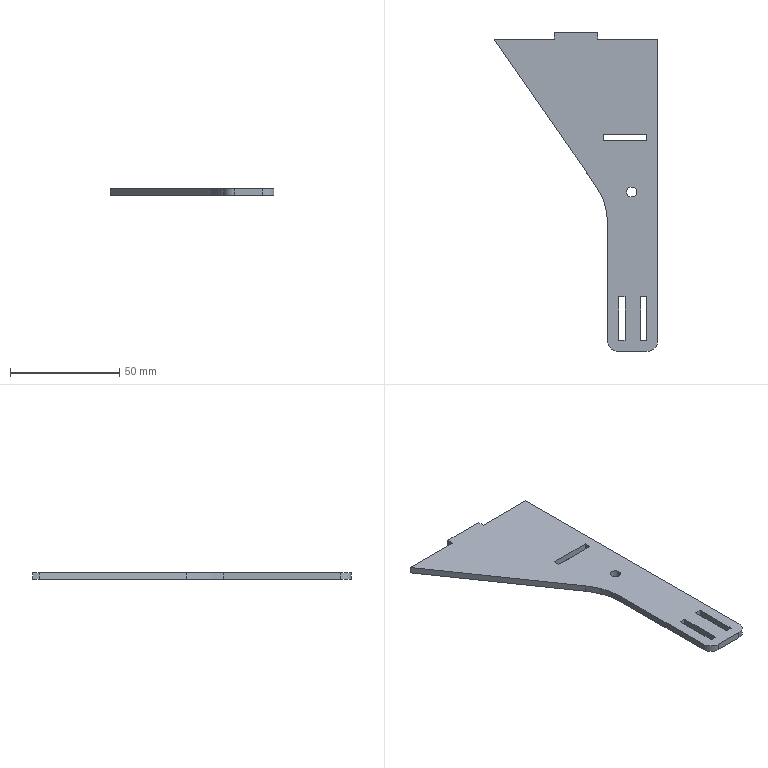Part | SolidWorks | features Fillet 2, Cut 1, Extrusion 1, ICE 1 | 1 solid | 28 faces | box 75 x 146 x 3 mm | volume 15319 mm3 | plane 23 | cylinder 5 | commonest cylinder face diameters 4.6 x2 10 x2 60 x1
STEP:
#1=CARTESIAN_POINT('',(-14.3,73.,0.));
#2=VERTEX_POINT('',#1);
#3=CARTESIAN_POINT('',(-9.7,73.,0.));
#4=VERTEX_POINT('',#3);
#5=CARTESIAN_POINT('',(-12.,73.,0.));
#6=DIRECTION('',(0.,0.,1.));
#7=DIRECTION('',(1.,0.,0.));
#8=AXIS2_PLACEMENT_3D('',#5,#6,#7);
#9=CIRCLE('',#8,2.3);
#10=EDGE_CURVE('',#2,#4,#9,.T.);
#11=ORIENTED_EDGE('',*,*,#10,.F.);
#12=CARTESIAN_POINT('',(-14.3,73.,3.));
#13=VERTEX_POINT('',#12);
#14=CARTESIAN_POINT('',(-14.3,73.,-7.));
#15=DIRECTION('',(0.,0.,1.));
#16=VECTOR('',#15,1000.);
#17=LINE('',#14,#16);
#18=EDGE_CURVE('',#2,#13,#17,.T.);
#19=ORIENTED_EDGE('',*,*,#18,.T.);
#20=CARTESIAN_POINT('',(-9.7,73.,3.));
#21=VERTEX_POINT('',#20);
#22=CARTESIAN_POINT('',(-12.,73.,3.));
#23=DIRECTION('',(0.,0.,1.));
#24=DIRECTION('',(1.,0.,0.));
#25=AXIS2_PLACEMENT_3D('',#22,#23,#24);
#26=CIRCLE('',#25,2.3);
#27=EDGE_CURVE('',#13,#21,#26,.T.);
#28=ORIENTED_EDGE('',*,*,#27,.T.);
#29=CARTESIAN_POINT('',(-9.7,73.,-7.));
#30=DIRECTION('',(0.,0.,1.));
#31=VECTOR('',#30,1000.);
#32=LINE('',#29,#31);
#33=EDGE_CURVE('',#4,#21,#32,.T.);
#34=ORIENTED_EDGE('',*,*,#33,.F.);
#35=EDGE_LOOP('',(#11,#19,#28,#34));
#36=FACE_OUTER_BOUND('',#35,.T.);
#37=CARTESIAN_POINT('',(-12.,73.,-7.));
#38=DIRECTION('',(0.,0.,1.));
#39=DIRECTION('',(1.,0.,0.));
#40=AXIS2_PLACEMENT_3D('',#37,#38,#39);
#41=CYLINDRICAL_SURFACE('',#40,2.3);
#42=ADVANCED_FACE('',(#36),#41,.F.);
#43=CARTESIAN_POINT('',(-5.,99.45,3.));
#44=VERTEX_POINT('',#43);
#45=CARTESIAN_POINT('',(-5.,96.55,3.));
#46=VERTEX_POINT('',#45);
#47=CARTESIAN_POINT('',(-5.,99.45,3.));
#48=DIRECTION('',(0.,-1.,0.));
#49=VECTOR('',#48,1000.);
#50=LINE('',#47,#49);
#51=EDGE_CURVE('',#44,#46,#50,.T.);
#52=ORIENTED_EDGE('',*,*,#51,.T.);
#53=CARTESIAN_POINT('',(-25.,96.55,3.));
#54=VERTEX_POINT('',#53);
#55=CARTESIAN_POINT('',(-5.,96.55,3.));
#56=DIRECTION('',(-1.,0.,0.));
#57=VECTOR('',#56,1000.);
#58=LINE('',#55,#57);
#59=EDGE_CURVE('',#46,#54,#58,.T.);
#60=ORIENTED_EDGE('',*,*,#59,.T.);
#61=CARTESIAN_POINT('',(-25.,99.45,3.));
#62=VERTEX_POINT('',#61);
#63=CARTESIAN_POINT('',(-25.,99.45,3.));
#64=DIRECTION('',(0.,1.,0.));
#65=VECTOR('',#64,1000.);
#66=LINE('',#63,#65);
#67=EDGE_CURVE('',#54,#62,#66,.T.);
#68=ORIENTED_EDGE('',*,*,#67,.T.);
#69=CARTESIAN_POINT('',(-5.,99.45,3.));
#70=DIRECTION('',(1.,0.,0.));
#71=VECTOR('',#70,1000.);
#72=LINE('',#69,#71);
#73=EDGE_CURVE('',#62,#44,#72,.T.);
#74=ORIENTED_EDGE('',*,*,#73,.T.);
#75=EDGE_LOOP('',(#52,#60,#68,#74));
#76=FACE_BOUND('',#75,.T.);
#77=CARTESIAN_POINT('',(-12.,73.,3.));
#78=DIRECTION('',(0.,0.,1.));
#79=DIRECTION('',(1.,0.,0.));
#80=AXIS2_PLACEMENT_3D('',#77,#78,#79);
#81=CIRCLE('',#80,2.3);
#82=EDGE_CURVE('',#21,#13,#81,.T.);
#83=ORIENTED_EDGE('',*,*,#82,.F.);
#84=ORIENTED_EDGE('',*,*,#27,.F.);
#85=EDGE_LOOP('',(#83,#84));
#86=FACE_BOUND('',#85,.T.);
#87=CARTESIAN_POINT('',(-17.95,5.,3.));
#88=VERTEX_POINT('',#87);
#89=CARTESIAN_POINT('',(-15.05,5.,3.));
#90=VERTEX_POINT('',#89);
#91=CARTESIAN_POINT('',(-17.95,5.,3.));
#92=DIRECTION('',(1.,0.,0.));
#93=VECTOR('',#92,1000.);
#94=LINE('',#91,#93);
#95=EDGE_CURVE('',#88,#90,#94,.T.);
#96=ORIENTED_EDGE('',*,*,#95,.F.);
#97=CARTESIAN_POINT('',(-17.95,25.,3.));
#98=VERTEX_POINT('',#97);
#99=CARTESIAN_POINT('',(-17.95,25.,3.));
#100=DIRECTION('',(0.,-1.,0.));
#101=VECTOR('',#100,1000.);
#102=LINE('',#99,#101);
#103=EDGE_CURVE('',#98,#88,#102,.T.);
#104=ORIENTED_EDGE('',*,*,#103,.F.);
#105=CARTESIAN_POINT('',(-15.05,25.,3.));
#106=VERTEX_POINT('',#105);
#107=CARTESIAN_POINT('',(-17.95,25.,3.));
#108=DIRECTION('',(-1.,0.,0.));
#109=VECTOR('',#108,1000.);
#110=LINE('',#107,#109);
#111=EDGE_CURVE('',#106,#98,#110,.T.);
#112=ORIENTED_EDGE('',*,*,#111,.F.);
#113=CARTESIAN_POINT('',(-15.05,25.,3.));
#114=DIRECTION('',(0.,1.,0.));
#115=VECTOR('',#114,1000.);
#116=LINE('',#113,#115);
#117=EDGE_CURVE('',#90,#106,#116,.T.);
#118=ORIENTED_EDGE('',*,*,#117,.F.);
#119=EDGE_LOOP('',(#96,#104,#112,#118));
#120=FACE_BOUND('',#119,.T.);
#121=CARTESIAN_POINT('',(-18.,0.,3.));
#122=VERTEX_POINT('',#121);
#123=CARTESIAN_POINT('',(-5.,0.,3.));
#124=VERTEX_POINT('',#123);
#125=CARTESIAN_POINT('',(0.,0.,3.));
#126=DIRECTION('',(1.,0.,0.));
#127=VECTOR('',#126,1000.);
#128=LINE('',#125,#127);
#129=EDGE_CURVE('',#122,#124,#128,.T.);
#130=ORIENTED_EDGE('',*,*,#129,.T.);
#131=CARTESIAN_POINT('',(0.,5.,3.));
#132=VERTEX_POINT('',#131);
#133=CARTESIAN_POINT('',(-5.,5.,3.));
#134=DIRECTION('',(0.,0.,1.));
#135=DIRECTION('',(1.,0.,0.));
#136=AXIS2_PLACEMENT_3D('',#133,#134,#135);
#137=CIRCLE('',#136,5.);
#138=EDGE_CURVE('',#124,#132,#137,.T.);
#139=ORIENTED_EDGE('',*,*,#138,.T.);
#140=CARTESIAN_POINT('',(0.,143.,3.));
#141=VERTEX_POINT('',#140);
#142=CARTESIAN_POINT('',(0.,0.,3.));
#143=DIRECTION('',(0.,1.,0.));
#144=VECTOR('',#143,1000.);
#145=LINE('',#142,#144);
#146=EDGE_CURVE('',#132,#141,#145,.T.);
#147=ORIENTED_EDGE('',*,*,#146,.T.);
#148=CARTESIAN_POINT('',(-27.5,143.,3.));
#149=VERTEX_POINT('',#148);
#150=CARTESIAN_POINT('',(0.,143.,3.));
#151=DIRECTION('',(-1.,0.,0.));
#152=VECTOR('',#151,1000.);
#153=LINE('',#150,#152);
#154=EDGE_CURVE('',#141,#149,#153,.T.);
#155=ORIENTED_EDGE('',*,*,#154,.T.);
#156=CARTESIAN_POINT('',(-27.5,146.,3.));
#157=VERTEX_POINT('',#156);
#158=CARTESIAN_POINT('',(-27.5,143.,3.));
#159=DIRECTION('',(0.,1.,0.));
#160=VECTOR('',#159,1000.);
#161=LINE('',#158,#160);
#162=EDGE_CURVE('',#149,#157,#161,.T.);
#163=ORIENTED_EDGE('',*,*,#162,.T.);
#164=CARTESIAN_POINT('',(-47.5,146.,3.));
#165=VERTEX_POINT('',#164);
#166=CARTESIAN_POINT('',(-47.5,146.,3.));
#167=DIRECTION('',(-1.,0.,0.));
#168=VECTOR('',#167,1000.);
#169=LINE('',#166,#168);
#170=EDGE_CURVE('',#157,#165,#169,.T.);
#171=ORIENTED_EDGE('',*,*,#170,.T.);
#172=CARTESIAN_POINT('',(-47.5,143.,3.));
#173=VERTEX_POINT('',#172);
#174=CARTESIAN_POINT('',(-47.5,143.,3.));
#175=DIRECTION('',(0.,-1.,0.));
#176=VECTOR('',#175,1000.);
#177=LINE('',#174,#176);
#178=EDGE_CURVE('',#165,#173,#177,.T.);
#179=ORIENTED_EDGE('',*,*,#178,.T.);
#180=CARTESIAN_POINT('',(-75.,143.,3.));
#181=VERTEX_POINT('',#180);
#182=CARTESIAN_POINT('',(-75.,143.,3.));
#183=DIRECTION('',(-1.,0.,0.));
#184=VECTOR('',#183,1000.);
#185=LINE('',#182,#184);
#186=EDGE_CURVE('',#173,#181,#185,.T.);
#187=ORIENTED_EDGE('',*,*,#186,.T.);
#188=CARTESIAN_POINT('',(-28.346,75.711,3.));
#189=VERTEX_POINT('',#188);
#190=CARTESIAN_POINT('',(-23.,68.,3.));
#191=DIRECTION('',(0.5698,-0.8218,0.));
#192=VECTOR('',#191,1000.);
#193=LINE('',#190,#192);
#194=EDGE_CURVE('',#181,#189,#193,.T.);
#195=ORIENTED_EDGE('',*,*,#194,.T.);
#196=CARTESIAN_POINT('',(-23.,58.617,3.));
#197=VERTEX_POINT('',#196);
#198=CARTESIAN_POINT('',(-53.,58.617,3.));
#199=DIRECTION('',(0.,0.,-1.));
#200=DIRECTION('',(1.,0.,0.));
#201=AXIS2_PLACEMENT_3D('',#198,#199,#200);
#202=CIRCLE('',#201,30.);
#203=EDGE_CURVE('',#189,#197,#202,.T.);
#204=ORIENTED_EDGE('',*,*,#203,.T.);
#205=CARTESIAN_POINT('',(-23.,5.,3.));
#206=VERTEX_POINT('',#205);
#207=CARTESIAN_POINT('',(-23.,0.,3.));
#208=DIRECTION('',(0.,-1.,0.));
#209=VECTOR('',#208,1000.);
#210=LINE('',#207,#209);
#211=EDGE_CURVE('',#197,#206,#210,.T.);
#212=ORIENTED_EDGE('',*,*,#211,.T.);
#213=CARTESIAN_POINT('',(-18.,5.,3.));
#214=DIRECTION('',(0.,0.,1.));
#215=DIRECTION('',(1.,0.,0.));
#216=AXIS2_PLACEMENT_3D('',#213,#214,#215);
#217=CIRCLE('',#216,5.);
#218=EDGE_CURVE('',#206,#122,#217,.T.);
#219=ORIENTED_EDGE('',*,*,#218,.T.);
#220=EDGE_LOOP('',(#130,#139,#147,#155,#163,#171,#179,#187,#195,#204,#212,#219));
#221=FACE_OUTER_BOUND('',#220,.T.);
#222=CARTESIAN_POINT('',(-7.95,5.,3.));
#223=VERTEX_POINT('',#222);
#224=CARTESIAN_POINT('',(-5.05,5.,3.));
#225=VERTEX_POINT('',#224);
#226=CARTESIAN_POINT('',(-7.95,5.,3.));
#227=DIRECTION('',(1.,0.,0.));
#228=VECTOR('',#227,1000.);
#229=LINE('',#226,#228);
#230=EDGE_CURVE('',#223,#225,#229,.T.);
#231=ORIENTED_EDGE('',*,*,#230,.F.);
#232=CARTESIAN_POINT('',(-7.95,25.,3.));
#233=VERTEX_POINT('',#232);
#234=CARTESIAN_POINT('',(-7.95,5.,3.));
#235=DIRECTION('',(0.,-1.,0.));
#236=VECTOR('',#235,1000.);
#237=LINE('',#234,#236);
#238=EDGE_CURVE('',#233,#223,#237,.T.);
#239=ORIENTED_EDGE('',*,*,#238,.F.);
#240=CARTESIAN_POINT('',(-5.05,25.,3.));
#241=VERTEX_POINT('',#240);
#242=CARTESIAN_POINT('',(-7.95,25.,3.));
#243=DIRECTION('',(-1.,0.,0.));
#244=VECTOR('',#243,1000.);
#245=LINE('',#242,#244);
#246=EDGE_CURVE('',#241,#233,#245,.T.);
#247=ORIENTED_EDGE('',*,*,#246,.F.);
#248=CARTESIAN_POINT('',(-5.05,5.,3.));
#249=DIRECTION('',(0.,1.,0.));
#250=VECTOR('',#249,1000.);
#251=LINE('',#248,#250);
#252=EDGE_CURVE('',#225,#241,#251,.T.);
#253=ORIENTED_EDGE('',*,*,#252,.F.);
#254=EDGE_LOOP('',(#231,#239,#247,#253));
#255=FACE_BOUND('',#254,.T.);
#256=CARTESIAN_POINT('',(0.,0.,3.));
#257=DIRECTION('',(0.,0.,1.));
#258=DIRECTION('',(1.,0.,0.));
#259=AXIS2_PLACEMENT_3D('',#256,#257,#258);
#260=PLANE('',#259);
#261=ADVANCED_FACE('',(#76,#86,#120,#221,#255),#260,.T.);
#262=CARTESIAN_POINT('',(-5.,96.55,0.));
#263=VERTEX_POINT('',#262);
#264=CARTESIAN_POINT('',(-25.,96.55,0.));
#265=VERTEX_POINT('',#264);
#266=CARTESIAN_POINT('',(-5.,96.55,0.));
#267=DIRECTION('',(-1.,0.,0.));
#268=VECTOR('',#267,1000.);
#269=LINE('',#266,#268);
#270=EDGE_CURVE('',#263,#265,#269,.T.);
#271=ORIENTED_EDGE('',*,*,#270,.F.);
#272=CARTESIAN_POINT('',(-5.,99.45,0.));
#273=VERTEX_POINT('',#272);
#274=CARTESIAN_POINT('',(-5.,99.45,0.));
#275=DIRECTION('',(0.,-1.,0.));
#276=VECTOR('',#275,1000.);
#277=LINE('',#274,#276);
#278=EDGE_CURVE('',#273,#263,#277,.T.);
#279=ORIENTED_EDGE('',*,*,#278,.F.);
#280=CARTESIAN_POINT('',(-25.,99.45,0.));
#281=VERTEX_POINT('',#280);
#282=CARTESIAN_POINT('',(-5.,99.45,0.));
#283=DIRECTION('',(1.,0.,0.));
#284=VECTOR('',#283,1000.);
#285=LINE('',#282,#284);
#286=EDGE_CURVE('',#281,#273,#285,.T.);
#287=ORIENTED_EDGE('',*,*,#286,.F.);
#288=CARTESIAN_POINT('',(-25.,99.45,0.));
#289=DIRECTION('',(0.,1.,0.));
#290=VECTOR('',#289,1000.);
#291=LINE('',#288,#290);
#292=EDGE_CURVE('',#265,#281,#291,.T.);
#293=ORIENTED_EDGE('',*,*,#292,.F.);
#294=EDGE_LOOP('',(#271,#279,#287,#293));
#295=FACE_BOUND('',#294,.T.);
#296=CARTESIAN_POINT('',(-12.,73.,0.));
#297=DIRECTION('',(0.,0.,1.));
#298=DIRECTION('',(1.,0.,0.));
#299=AXIS2_PLACEMENT_3D('',#296,#297,#298);
#300=CIRCLE('',#299,2.3);
#301=EDGE_CURVE('',#4,#2,#300,.T.);
#302=ORIENTED_EDGE('',*,*,#301,.T.);
#303=ORIENTED_EDGE('',*,*,#10,.T.);
#304=EDGE_LOOP('',(#302,#303));
#305=FACE_BOUND('',#304,.T.);
#306=CARTESIAN_POINT('',(-17.95,25.,0.));
#307=VERTEX_POINT('',#306);
#308=CARTESIAN_POINT('',(-17.95,5.,0.));
#309=VERTEX_POINT('',#308);
#310=CARTESIAN_POINT('',(-17.95,25.,0.));
#311=DIRECTION('',(0.,-1.,0.));
#312=VECTOR('',#311,1000.);
#313=LINE('',#310,#312);
#314=EDGE_CURVE('',#307,#309,#313,.T.);
#315=ORIENTED_EDGE('',*,*,#314,.T.);
#316=CARTESIAN_POINT('',(-15.05,5.,0.));
#317=VERTEX_POINT('',#316);
#318=CARTESIAN_POINT('',(-17.95,5.,0.));
#319=DIRECTION('',(1.,0.,0.));
#320=VECTOR('',#319,1000.);
#321=LINE('',#318,#320);
#322=EDGE_CURVE('',#309,#317,#321,.T.);
#323=ORIENTED_EDGE('',*,*,#322,.T.);
#324=CARTESIAN_POINT('',(-15.05,25.,0.));
#325=VERTEX_POINT('',#324);
#326=CARTESIAN_POINT('',(-15.05,25.,0.));
#327=DIRECTION('',(0.,1.,0.));
#328=VECTOR('',#327,1000.);
#329=LINE('',#326,#328);
#330=EDGE_CURVE('',#317,#325,#329,.T.);
#331=ORIENTED_EDGE('',*,*,#330,.T.);
#332=CARTESIAN_POINT('',(-17.95,25.,0.));
#333=DIRECTION('',(-1.,0.,0.));
#334=VECTOR('',#333,1000.);
#335=LINE('',#332,#334);
#336=EDGE_CURVE('',#325,#307,#335,.T.);
#337=ORIENTED_EDGE('',*,*,#336,.T.);
#338=EDGE_LOOP('',(#315,#323,#331,#337));
#339=FACE_BOUND('',#338,.T.);
#340=CARTESIAN_POINT('',(0.,5.,0.));
#341=VERTEX_POINT('',#340);
#342=CARTESIAN_POINT('',(0.,143.,0.));
#343=VERTEX_POINT('',#342);
#344=CARTESIAN_POINT('',(0.,0.,0.));
#345=DIRECTION('',(0.,1.,0.));
#346=VECTOR('',#345,1000.);
#347=LINE('',#344,#346);
#348=EDGE_CURVE('',#341,#343,#347,.T.);
#349=ORIENTED_EDGE('',*,*,#348,.F.);
#350=CARTESIAN_POINT('',(-5.,0.,0.));
#351=VERTEX_POINT('',#350);
#352=CARTESIAN_POINT('',(-5.,5.,0.));
#353=DIRECTION('',(0.,0.,-1.));
#354=DIRECTION('',(1.,0.,0.));
#355=AXIS2_PLACEMENT_3D('',#352,#353,#354);
#356=CIRCLE('',#355,5.);
#357=EDGE_CURVE('',#341,#351,#356,.T.);
#358=ORIENTED_EDGE('',*,*,#357,.T.);
#359=CARTESIAN_POINT('',(-18.,0.,0.));
#360=VERTEX_POINT('',#359);
#361=CARTESIAN_POINT('',(0.,0.,0.));
#362=DIRECTION('',(1.,0.,0.));
#363=VECTOR('',#362,1000.);
#364=LINE('',#361,#363);
#365=EDGE_CURVE('',#360,#351,#364,.T.);
#366=ORIENTED_EDGE('',*,*,#365,.F.);
#367=CARTESIAN_POINT('',(-23.,5.,0.));
#368=VERTEX_POINT('',#367);
#369=CARTESIAN_POINT('',(-18.,5.,0.));
#370=DIRECTION('',(0.,0.,-1.));
#371=DIRECTION('',(1.,0.,0.));
#372=AXIS2_PLACEMENT_3D('',#369,#370,#371);
#373=CIRCLE('',#372,5.);
#374=EDGE_CURVE('',#360,#368,#373,.T.);
#375=ORIENTED_EDGE('',*,*,#374,.T.);
#376=CARTESIAN_POINT('',(-23.,58.617,0.));
#377=VERTEX_POINT('',#376);
#378=CARTESIAN_POINT('',(-23.,0.,0.));
#379=DIRECTION('',(0.,-1.,0.));
#380=VECTOR('',#379,1000.);
#381=LINE('',#378,#380);
#382=EDGE_CURVE('',#377,#368,#381,.T.);
#383=ORIENTED_EDGE('',*,*,#382,.F.);
#384=CARTESIAN_POINT('',(-28.346,75.711,0.));
#385=VERTEX_POINT('',#384);
#386=CARTESIAN_POINT('',(-53.,58.617,0.));
#387=DIRECTION('',(0.,0.,1.));
#388=DIRECTION('',(1.,0.,0.));
#389=AXIS2_PLACEMENT_3D('',#386,#387,#388);
#390=CIRCLE('',#389,30.);
#391=EDGE_CURVE('',#377,#385,#390,.T.);
#392=ORIENTED_EDGE('',*,*,#391,.T.);
#393=CARTESIAN_POINT('',(-75.,143.,0.));
#394=VERTEX_POINT('',#393);
#395=CARTESIAN_POINT('',(-23.,68.,0.));
#396=DIRECTION('',(0.5698,-0.8218,0.));
#397=VECTOR('',#396,1000.);
#398=LINE('',#395,#397);
#399=EDGE_CURVE('',#394,#385,#398,.T.);
#400=ORIENTED_EDGE('',*,*,#399,.F.);
#401=CARTESIAN_POINT('',(-47.5,143.,0.));
#402=VERTEX_POINT('',#401);
#403=CARTESIAN_POINT('',(-75.,143.,0.));
#404=DIRECTION('',(-1.,0.,0.));
#405=VECTOR('',#404,1000.);
#406=LINE('',#403,#405);
#407=EDGE_CURVE('',#402,#394,#406,.T.);
#408=ORIENTED_EDGE('',*,*,#407,.F.);
#409=CARTESIAN_POINT('',(-47.5,146.,0.));
#410=VERTEX_POINT('',#409);
#411=CARTESIAN_POINT('',(-47.5,143.,0.));
#412=DIRECTION('',(0.,-1.,0.));
#413=VECTOR('',#412,1000.);
#414=LINE('',#411,#413);
#415=EDGE_CURVE('',#410,#402,#414,.T.);
#416=ORIENTED_EDGE('',*,*,#415,.F.);
#417=CARTESIAN_POINT('',(-27.5,146.,0.));
#418=VERTEX_POINT('',#417);
#419=CARTESIAN_POINT('',(-47.5,146.,0.));
#420=DIRECTION('',(-1.,0.,0.));
#421=VECTOR('',#420,1000.);
#422=LINE('',#419,#421);
#423=EDGE_CURVE('',#418,#410,#422,.T.);
#424=ORIENTED_EDGE('',*,*,#423,.F.);
#425=CARTESIAN_POINT('',(-27.5,143.,0.));
#426=VERTEX_POINT('',#425);
#427=CARTESIAN_POINT('',(-27.5,143.,0.));
#428=DIRECTION('',(0.,1.,0.));
#429=VECTOR('',#428,1000.);
#430=LINE('',#427,#429);
#431=EDGE_CURVE('',#426,#418,#430,.T.);
#432=ORIENTED_EDGE('',*,*,#431,.F.);
#433=CARTESIAN_POINT('',(0.,143.,0.));
#434=DIRECTION('',(-1.,0.,0.));
#435=VECTOR('',#434,1000.);
#436=LINE('',#433,#435);
#437=EDGE_CURVE('',#343,#426,#436,.T.);
#438=ORIENTED_EDGE('',*,*,#437,.F.);
#439=EDGE_LOOP('',(#349,#358,#366,#375,#383,#392,#400,#408,#416,#424,#432,#438));
#440=FACE_OUTER_BOUND('',#439,.T.);
#441=CARTESIAN_POINT('',(-7.95,25.,0.));
#442=VERTEX_POINT('',#441);
#443=CARTESIAN_POINT('',(-7.95,5.,0.));
#444=VERTEX_POINT('',#443);
#445=CARTESIAN_POINT('',(-7.95,5.,0.));
#446=DIRECTION('',(0.,-1.,0.));
#447=VECTOR('',#446,1000.);
#448=LINE('',#445,#447);
#449=EDGE_CURVE('',#442,#444,#448,.T.);
#450=ORIENTED_EDGE('',*,*,#449,.T.);
#451=CARTESIAN_POINT('',(-5.05,5.,0.));
#452=VERTEX_POINT('',#451);
#453=CARTESIAN_POINT('',(-7.95,5.,0.));
#454=DIRECTION('',(1.,0.,0.));
#455=VECTOR('',#454,1000.);
#456=LINE('',#453,#455);
#457=EDGE_CURVE('',#444,#452,#456,.T.);
#458=ORIENTED_EDGE('',*,*,#457,.T.);
#459=CARTESIAN_POINT('',(-5.05,25.,0.));
#460=VERTEX_POINT('',#459);
#461=CARTESIAN_POINT('',(-5.05,5.,0.));
#462=DIRECTION('',(0.,1.,0.));
#463=VECTOR('',#462,1000.);
#464=LINE('',#461,#463);
#465=EDGE_CURVE('',#452,#460,#464,.T.);
#466=ORIENTED_EDGE('',*,*,#465,.T.);
#467=CARTESIAN_POINT('',(-7.95,25.,0.));
#468=DIRECTION('',(-1.,0.,0.));
#469=VECTOR('',#468,1000.);
#470=LINE('',#467,#469);
#471=EDGE_CURVE('',#460,#442,#470,.T.);
#472=ORIENTED_EDGE('',*,*,#471,.T.);
#473=EDGE_LOOP('',(#450,#458,#466,#472));
#474=FACE_BOUND('',#473,.T.);
#475=CARTESIAN_POINT('',(0.,0.,0.));
#476=DIRECTION('',(0.,0.,1.));
#477=DIRECTION('',(1.,0.,0.));
#478=AXIS2_PLACEMENT_3D('',#475,#476,#477);
#479=PLANE('',#478);
#480=ADVANCED_FACE('',(#295,#305,#339,#440,#474),#479,.F.);
#481=ORIENTED_EDGE('',*,*,#146,.F.);
#482=CARTESIAN_POINT('',(0.,5.,3.));
#483=DIRECTION('',(0.,0.,-1.));
#484=VECTOR('',#483,1000.);
#485=LINE('',#482,#484);
#486=EDGE_CURVE('',#132,#341,#485,.T.);
#487=ORIENTED_EDGE('',*,*,#486,.T.);
#488=ORIENTED_EDGE('',*,*,#348,.T.);
#489=CARTESIAN_POINT('',(0.,143.,3.));
#490=DIRECTION('',(0.,0.,-1.));
#491=VECTOR('',#490,1000.);
#492=LINE('',#489,#491);
#493=EDGE_CURVE('',#141,#343,#492,.T.);
#494=ORIENTED_EDGE('',*,*,#493,.F.);
#495=EDGE_LOOP('',(#481,#487,#488,#494));
#496=FACE_OUTER_BOUND('',#495,.T.);
#497=CARTESIAN_POINT('',(0.,0.,3.));
#498=DIRECTION('',(-1.,0.,0.));
#499=DIRECTION('',(0.,0.,1.));
#500=AXIS2_PLACEMENT_3D('',#497,#498,#499);
#501=PLANE('',#500);
#502=ADVANCED_FACE('',(#496),#501,.F.);
#503=ORIENTED_EDGE('',*,*,#437,.T.);
#504=CARTESIAN_POINT('',(-27.5,143.,3.));
#505=DIRECTION('',(0.,0.,-1.));
#506=VECTOR('',#505,1000.);
#507=LINE('',#504,#506);
#508=EDGE_CURVE('',#149,#426,#507,.T.);
#509=ORIENTED_EDGE('',*,*,#508,.F.);
#510=ORIENTED_EDGE('',*,*,#154,.F.);
#511=ORIENTED_EDGE('',*,*,#493,.T.);
#512=EDGE_LOOP('',(#503,#509,#510,#511));
#513=FACE_OUTER_BOUND('',#512,.T.);
#514=CARTESIAN_POINT('',(0.,143.,3.));
#515=DIRECTION('',(0.,-1.,0.));
#516=DIRECTION('',(0.,0.,-1.));
#517=AXIS2_PLACEMENT_3D('',#514,#515,#516);
#518=PLANE('',#517);
#519=ADVANCED_FACE('',(#513),#518,.F.);
#520=ORIENTED_EDGE('',*,*,#431,.T.);
#521=CARTESIAN_POINT('',(-27.5,146.,3.));
#522=DIRECTION('',(0.,0.,-1.));
#523=VECTOR('',#522,1000.);
#524=LINE('',#521,#523);
#525=EDGE_CURVE('',#157,#418,#524,.T.);
#526=ORIENTED_EDGE('',*,*,#525,.F.);
#527=ORIENTED_EDGE('',*,*,#162,.F.);
#528=ORIENTED_EDGE('',*,*,#508,.T.);
#529=EDGE_LOOP('',(#520,#526,#527,#528));
#530=FACE_OUTER_BOUND('',#529,.T.);
#531=CARTESIAN_POINT('',(-27.5,143.,3.));
#532=DIRECTION('',(-1.,0.,0.));
#533=DIRECTION('',(0.,0.,1.));
#534=AXIS2_PLACEMENT_3D('',#531,#532,#533);
#535=PLANE('',#534);
#536=ADVANCED_FACE('',(#530),#535,.F.);
#537=ORIENTED_EDGE('',*,*,#423,.T.);
#538=CARTESIAN_POINT('',(-47.5,146.,3.));
#539=DIRECTION('',(0.,0.,-1.));
#540=VECTOR('',#539,1000.);
#541=LINE('',#538,#540);
#542=EDGE_CURVE('',#165,#410,#541,.T.);
#543=ORIENTED_EDGE('',*,*,#542,.F.);
#544=ORIENTED_EDGE('',*,*,#170,.F.);
#545=ORIENTED_EDGE('',*,*,#525,.T.);
#546=EDGE_LOOP('',(#537,#543,#544,#545));
#547=FACE_OUTER_BOUND('',#546,.T.);
#548=CARTESIAN_POINT('',(-47.5,146.,3.));
#549=DIRECTION('',(0.,-1.,0.));
#550=DIRECTION('',(0.,0.,-1.));
#551=AXIS2_PLACEMENT_3D('',#548,#549,#550);
#552=PLANE('',#551);
#553=ADVANCED_FACE('',(#547),#552,.F.);
#554=ORIENTED_EDGE('',*,*,#415,.T.);
#555=CARTESIAN_POINT('',(-47.5,143.,3.));
#556=DIRECTION('',(0.,0.,-1.));
#557=VECTOR('',#556,1000.);
#558=LINE('',#555,#557);
#559=EDGE_CURVE('',#173,#402,#558,.T.);
#560=ORIENTED_EDGE('',*,*,#559,.F.);
#561=ORIENTED_EDGE('',*,*,#178,.F.);
#562=ORIENTED_EDGE('',*,*,#542,.T.);
#563=EDGE_LOOP('',(#554,#560,#561,#562));
#564=FACE_OUTER_BOUND('',#563,.T.);
#565=CARTESIAN_POINT('',(-47.5,143.,3.));
#566=DIRECTION('',(1.,0.,0.));
#567=DIRECTION('',(0.,0.,-1.));
#568=AXIS2_PLACEMENT_3D('',#565,#566,#567);
#569=PLANE('',#568);
#570=ADVANCED_FACE('',(#564),#569,.F.);
#571=ORIENTED_EDGE('',*,*,#407,.T.);
#572=CARTESIAN_POINT('',(-75.,143.,3.));
#573=DIRECTION('',(0.,0.,-1.));
#574=VECTOR('',#573,1000.);
#575=LINE('',#572,#574);
#576=EDGE_CURVE('',#181,#394,#575,.T.);
#577=ORIENTED_EDGE('',*,*,#576,.F.);
#578=ORIENTED_EDGE('',*,*,#186,.F.);
#579=ORIENTED_EDGE('',*,*,#559,.T.);
#580=EDGE_LOOP('',(#571,#577,#578,#579));
#581=FACE_OUTER_BOUND('',#580,.T.);
#582=CARTESIAN_POINT('',(-75.,143.,3.));
#583=DIRECTION('',(0.,-1.,0.));
#584=DIRECTION('',(0.,0.,-1.));
#585=AXIS2_PLACEMENT_3D('',#582,#583,#584);
#586=PLANE('',#585);
#587=ADVANCED_FACE('',(#581),#586,.F.);
#588=ORIENTED_EDGE('',*,*,#399,.T.);
#589=CARTESIAN_POINT('',(-28.346,75.711,3.));
#590=DIRECTION('',(0.,0.,1.));
#591=VECTOR('',#590,1000.);
#592=LINE('',#589,#591);
#593=EDGE_CURVE('',#385,#189,#592,.T.);
#594=ORIENTED_EDGE('',*,*,#593,.T.);
#595=ORIENTED_EDGE('',*,*,#194,.F.);
#596=ORIENTED_EDGE('',*,*,#576,.T.);
#597=EDGE_LOOP('',(#588,#594,#595,#596));
#598=FACE_OUTER_BOUND('',#597,.T.);
#599=CARTESIAN_POINT('',(-23.,68.,3.));
#600=DIRECTION('',(0.8218,0.5698,0.));
#601=DIRECTION('',(-0.5698,0.8218,0.));
#602=AXIS2_PLACEMENT_3D('',#599,#600,#601);
#603=PLANE('',#602);
#604=ADVANCED_FACE('',(#598),#603,.F.);
#605=ORIENTED_EDGE('',*,*,#211,.F.);
#606=CARTESIAN_POINT('',(-23.,58.617,0.));
#607=DIRECTION('',(0.,0.,-1.));
#608=VECTOR('',#607,1000.);
#609=LINE('',#606,#608);
#610=EDGE_CURVE('',#197,#377,#609,.T.);
#611=ORIENTED_EDGE('',*,*,#610,.T.);
#612=ORIENTED_EDGE('',*,*,#382,.T.);
#613=CARTESIAN_POINT('',(-23.,5.,3.));
#614=DIRECTION('',(0.,0.,1.));
#615=VECTOR('',#614,1000.);
#616=LINE('',#613,#615);
#617=EDGE_CURVE('',#368,#206,#616,.T.);
#618=ORIENTED_EDGE('',*,*,#617,.T.);
#619=EDGE_LOOP('',(#605,#611,#612,#618));
#620=FACE_OUTER_BOUND('',#619,.T.);
#621=CARTESIAN_POINT('',(-23.,0.,3.));
#622=DIRECTION('',(1.,0.,0.));
#623=DIRECTION('',(0.,0.,-1.));
#624=AXIS2_PLACEMENT_3D('',#621,#622,#623);
#625=PLANE('',#624);
#626=ADVANCED_FACE('',(#620),#625,.F.);
#627=ORIENTED_EDGE('',*,*,#365,.T.);
#628=CARTESIAN_POINT('',(-5.,0.,3.));
#629=DIRECTION('',(0.,0.,1.));
#630=VECTOR('',#629,1000.);
#631=LINE('',#628,#630);
#632=EDGE_CURVE('',#351,#124,#631,.T.);
#633=ORIENTED_EDGE('',*,*,#632,.T.);
#634=ORIENTED_EDGE('',*,*,#129,.F.);
#635=CARTESIAN_POINT('',(-18.,0.,3.));
#636=DIRECTION('',(0.,0.,-1.));
#637=VECTOR('',#636,1000.);
#638=LINE('',#635,#637);
#639=EDGE_CURVE('',#122,#360,#638,.T.);
#640=ORIENTED_EDGE('',*,*,#639,.T.);
#641=EDGE_LOOP('',(#627,#633,#634,#640));
#642=FACE_OUTER_BOUND('',#641,.T.);
#643=CARTESIAN_POINT('',(0.,0.,3.));
#644=DIRECTION('',(0.,1.,0.));
#645=DIRECTION('',(0.,0.,1.));
#646=AXIS2_PLACEMENT_3D('',#643,#644,#645);
#647=PLANE('',#646);
#648=ADVANCED_FACE('',(#642),#647,.F.);
#649=ORIENTED_EDGE('',*,*,#314,.F.);
#650=CARTESIAN_POINT('',(-17.95,25.,3.));
#651=DIRECTION('',(0.,0.,-1.));
#652=VECTOR('',#651,1000.);
#653=LINE('',#650,#652);
#654=EDGE_CURVE('',#98,#307,#653,.T.);
#655=ORIENTED_EDGE('',*,*,#654,.F.);
#656=ORIENTED_EDGE('',*,*,#103,.T.);
#657=CARTESIAN_POINT('',(-17.95,5.,3.));
#658=DIRECTION('',(0.,0.,-1.));
#659=VECTOR('',#658,1000.);
#660=LINE('',#657,#659);
#661=EDGE_CURVE('',#88,#309,#660,.T.);
#662=ORIENTED_EDGE('',*,*,#661,.T.);
#663=EDGE_LOOP('',(#649,#655,#656,#662));
#664=FACE_OUTER_BOUND('',#663,.T.);
#665=CARTESIAN_POINT('',(-17.95,25.,3.));
#666=DIRECTION('',(1.,0.,0.));
#667=DIRECTION('',(0.,1.,0.));
#668=AXIS2_PLACEMENT_3D('',#665,#666,#667);
#669=PLANE('',#668);
#670=ADVANCED_FACE('',(#664),#669,.T.);
#671=ORIENTED_EDGE('',*,*,#322,.F.);
#672=ORIENTED_EDGE('',*,*,#661,.F.);
#673=ORIENTED_EDGE('',*,*,#95,.T.);
#674=CARTESIAN_POINT('',(-15.05,5.,3.));
#675=DIRECTION('',(0.,0.,-1.));
#676=VECTOR('',#675,1000.);
#677=LINE('',#674,#676);
#678=EDGE_CURVE('',#90,#317,#677,.T.);
#679=ORIENTED_EDGE('',*,*,#678,.T.);
#680=EDGE_LOOP('',(#671,#672,#673,#679));
#681=FACE_OUTER_BOUND('',#680,.T.);
#682=CARTESIAN_POINT('',(-17.95,5.,3.));
#683=DIRECTION('',(0.,1.,0.));
#684=DIRECTION('',(-1.,0.,0.));
#685=AXIS2_PLACEMENT_3D('',#682,#683,#684);
#686=PLANE('',#685);
#687=ADVANCED_FACE('',(#681),#686,.T.);
#688=ORIENTED_EDGE('',*,*,#330,.F.);
#689=ORIENTED_EDGE('',*,*,#678,.F.);
#690=ORIENTED_EDGE('',*,*,#117,.T.);
#691=CARTESIAN_POINT('',(-15.05,25.,3.));
#692=DIRECTION('',(0.,0.,-1.));
#693=VECTOR('',#692,1000.);
#694=LINE('',#691,#693);
#695=EDGE_CURVE('',#106,#325,#694,.T.);
#696=ORIENTED_EDGE('',*,*,#695,.T.);
#697=EDGE_LOOP('',(#688,#689,#690,#696));
#698=FACE_OUTER_BOUND('',#697,.T.);
#699=CARTESIAN_POINT('',(-15.05,25.,3.));
#700=DIRECTION('',(-1.,0.,0.));
#701=DIRECTION('',(0.,-1.,0.));
#702=AXIS2_PLACEMENT_3D('',#699,#700,#701);
#703=PLANE('',#702);
#704=ADVANCED_FACE('',(#698),#703,.T.);
#705=ORIENTED_EDGE('',*,*,#336,.F.);
#706=ORIENTED_EDGE('',*,*,#695,.F.);
#707=ORIENTED_EDGE('',*,*,#111,.T.);
#708=ORIENTED_EDGE('',*,*,#654,.T.);
#709=EDGE_LOOP('',(#705,#706,#707,#708));
#710=FACE_OUTER_BOUND('',#709,.T.);
#711=CARTESIAN_POINT('',(-17.95,25.,3.));
#712=DIRECTION('',(0.,-1.,0.));
#713=DIRECTION('',(1.,0.,0.));
#714=AXIS2_PLACEMENT_3D('',#711,#712,#713);
#715=PLANE('',#714);
#716=ADVANCED_FACE('',(#710),#715,.T.);
#717=ORIENTED_EDGE('',*,*,#449,.F.);
#718=CARTESIAN_POINT('',(-7.95,25.,3.));
#719=DIRECTION('',(0.,0.,-1.));
#720=VECTOR('',#719,1000.);
#721=LINE('',#718,#720);
#722=EDGE_CURVE('',#233,#442,#721,.T.);
#723=ORIENTED_EDGE('',*,*,#722,.F.);
#724=ORIENTED_EDGE('',*,*,#238,.T.);
#725=CARTESIAN_POINT('',(-7.95,5.,3.));
#726=DIRECTION('',(0.,0.,-1.));
#727=VECTOR('',#726,1000.);
#728=LINE('',#725,#727);
#729=EDGE_CURVE('',#223,#444,#728,.T.);
#730=ORIENTED_EDGE('',*,*,#729,.T.);
#731=EDGE_LOOP('',(#717,#723,#724,#730));
#732=FACE_OUTER_BOUND('',#731,.T.);
#733=CARTESIAN_POINT('',(-7.95,5.,3.));
#734=DIRECTION('',(1.,0.,0.));
#735=DIRECTION('',(0.,1.,0.));
#736=AXIS2_PLACEMENT_3D('',#733,#734,#735);
#737=PLANE('',#736);
#738=ADVANCED_FACE('',(#732),#737,.T.);
#739=ORIENTED_EDGE('',*,*,#457,.F.);
#740=ORIENTED_EDGE('',*,*,#729,.F.);
#741=ORIENTED_EDGE('',*,*,#230,.T.);
#742=CARTESIAN_POINT('',(-5.05,5.,3.));
#743=DIRECTION('',(0.,0.,-1.));
#744=VECTOR('',#743,1000.);
#745=LINE('',#742,#744);
#746=EDGE_CURVE('',#225,#452,#745,.T.);
#747=ORIENTED_EDGE('',*,*,#746,.T.);
#748=EDGE_LOOP('',(#739,#740,#741,#747));
#749=FACE_OUTER_BOUND('',#748,.T.);
#750=CARTESIAN_POINT('',(-7.95,5.,3.));
#751=DIRECTION('',(0.,1.,0.));
#752=DIRECTION('',(-1.,0.,0.));
#753=AXIS2_PLACEMENT_3D('',#750,#751,#752);
#754=PLANE('',#753);
#755=ADVANCED_FACE('',(#749),#754,.T.);
#756=ORIENTED_EDGE('',*,*,#465,.F.);
#757=ORIENTED_EDGE('',*,*,#746,.F.);
#758=ORIENTED_EDGE('',*,*,#252,.T.);
#759=CARTESIAN_POINT('',(-5.05,25.,3.));
#760=DIRECTION('',(0.,0.,-1.));
#761=VECTOR('',#760,1000.);
#762=LINE('',#759,#761);
#763=EDGE_CURVE('',#241,#460,#762,.T.);
#764=ORIENTED_EDGE('',*,*,#763,.T.);
#765=EDGE_LOOP('',(#756,#757,#758,#764));
#766=FACE_OUTER_BOUND('',#765,.T.);
#767=CARTESIAN_POINT('',(-5.05,5.,3.));
#768=DIRECTION('',(-1.,0.,0.));
#769=DIRECTION('',(0.,-1.,0.));
#770=AXIS2_PLACEMENT_3D('',#767,#768,#769);
#771=PLANE('',#770);
#772=ADVANCED_FACE('',(#766),#771,.T.);
#773=ORIENTED_EDGE('',*,*,#471,.F.);
#774=ORIENTED_EDGE('',*,*,#763,.F.);
#775=ORIENTED_EDGE('',*,*,#246,.T.);
#776=ORIENTED_EDGE('',*,*,#722,.T.);
#777=EDGE_LOOP('',(#773,#774,#775,#776));
#778=FACE_OUTER_BOUND('',#777,.T.);
#779=CARTESIAN_POINT('',(-7.95,25.,3.));
#780=DIRECTION('',(0.,-1.,0.));
#781=DIRECTION('',(0.,0.,-1.));
#782=AXIS2_PLACEMENT_3D('',#779,#780,#781);
#783=PLANE('',#782);
#784=ADVANCED_FACE('',(#778),#783,.T.);
#785=ORIENTED_EDGE('',*,*,#138,.F.);
#786=ORIENTED_EDGE('',*,*,#632,.F.);
#787=ORIENTED_EDGE('',*,*,#357,.F.);
#788=ORIENTED_EDGE('',*,*,#486,.F.);
#789=EDGE_LOOP('',(#785,#786,#787,#788));
#790=FACE_OUTER_BOUND('',#789,.T.);
#791=CARTESIAN_POINT('',(-5.,5.,3.));
#792=DIRECTION('',(0.,0.,-1.));
#793=DIRECTION('',(-1.,0.,0.));
#794=AXIS2_PLACEMENT_3D('',#791,#792,#793);
#795=CYLINDRICAL_SURFACE('',#794,5.);
#796=ADVANCED_FACE('',(#790),#795,.T.);
#797=ORIENTED_EDGE('',*,*,#218,.F.);
#798=ORIENTED_EDGE('',*,*,#617,.F.);
#799=ORIENTED_EDGE('',*,*,#374,.F.);
#800=ORIENTED_EDGE('',*,*,#639,.F.);
#801=EDGE_LOOP('',(#797,#798,#799,#800));
#802=FACE_OUTER_BOUND('',#801,.T.);
#803=CARTESIAN_POINT('',(-18.,5.,3.));
#804=DIRECTION('',(0.,0.,-1.));
#805=DIRECTION('',(-1.,0.,0.));
#806=AXIS2_PLACEMENT_3D('',#803,#804,#805);
#807=CYLINDRICAL_SURFACE('',#806,5.);
#808=ADVANCED_FACE('',(#802),#807,.T.);
#809=ORIENTED_EDGE('',*,*,#203,.F.);
#810=ORIENTED_EDGE('',*,*,#593,.F.);
#811=ORIENTED_EDGE('',*,*,#391,.F.);
#812=ORIENTED_EDGE('',*,*,#610,.F.);
#813=EDGE_LOOP('',(#809,#810,#811,#812));
#814=FACE_OUTER_BOUND('',#813,.T.);
#815=CARTESIAN_POINT('',(-53.,58.617,3.));
#816=DIRECTION('',(0.,0.,1.));
#817=DIRECTION('',(1.,0.,0.));
#818=AXIS2_PLACEMENT_3D('',#815,#816,#817);
#819=CYLINDRICAL_SURFACE('',#818,30.);
#820=ADVANCED_FACE('',(#814),#819,.F.);
#821=ORIENTED_EDGE('',*,*,#18,.F.);
#822=ORIENTED_EDGE('',*,*,#301,.F.);
#823=ORIENTED_EDGE('',*,*,#33,.T.);
#824=ORIENTED_EDGE('',*,*,#82,.T.);
#825=EDGE_LOOP('',(#821,#822,#823,#824));
#826=FACE_OUTER_BOUND('',#825,.T.);
#827=CARTESIAN_POINT('',(-12.,73.,-7.));
#828=DIRECTION('',(0.,0.,1.));
#829=DIRECTION('',(1.,0.,0.));
#830=AXIS2_PLACEMENT_3D('',#827,#828,#829);
#831=CYLINDRICAL_SURFACE('',#830,2.3);
#832=ADVANCED_FACE('',(#826),#831,.F.);
#833=ORIENTED_EDGE('',*,*,#278,.T.);
#834=CARTESIAN_POINT('',(-5.,96.55,3.));
#835=DIRECTION('',(0.,0.,-1.));
#836=VECTOR('',#835,1000.);
#837=LINE('',#834,#836);
#838=EDGE_CURVE('',#46,#263,#837,.T.);
#839=ORIENTED_EDGE('',*,*,#838,.F.);
#840=ORIENTED_EDGE('',*,*,#51,.F.);
#841=CARTESIAN_POINT('',(-5.,99.45,3.));
#842=DIRECTION('',(0.,0.,-1.));
#843=VECTOR('',#842,1000.);
#844=LINE('',#841,#843);
#845=EDGE_CURVE('',#44,#273,#844,.T.);
#846=ORIENTED_EDGE('',*,*,#845,.T.);
#847=EDGE_LOOP('',(#833,#839,#840,#846));
#848=FACE_OUTER_BOUND('',#847,.T.);
#849=CARTESIAN_POINT('',(-5.,99.45,3.));
#850=DIRECTION('',(1.,0.,0.));
#851=DIRECTION('',(0.,0.,-1.));
#852=AXIS2_PLACEMENT_3D('',#849,#850,#851);
#853=PLANE('',#852);
#854=ADVANCED_FACE('',(#848),#853,.F.);
#855=ORIENTED_EDGE('',*,*,#286,.T.);
#856=ORIENTED_EDGE('',*,*,#845,.F.);
#857=ORIENTED_EDGE('',*,*,#73,.F.);
#858=CARTESIAN_POINT('',(-25.,99.45,3.));
#859=DIRECTION('',(0.,0.,-1.));
#860=VECTOR('',#859,1000.);
#861=LINE('',#858,#860);
#862=EDGE_CURVE('',#62,#281,#861,.T.);
#863=ORIENTED_EDGE('',*,*,#862,.T.);
#864=EDGE_LOOP('',(#855,#856,#857,#863));
#865=FACE_OUTER_BOUND('',#864,.T.);
#866=CARTESIAN_POINT('',(-5.,99.45,3.));
#867=DIRECTION('',(0.,1.,0.));
#868=DIRECTION('',(-1.,0.,0.));
#869=AXIS2_PLACEMENT_3D('',#866,#867,#868);
#870=PLANE('',#869);
#871=ADVANCED_FACE('',(#865),#870,.F.);
#872=ORIENTED_EDGE('',*,*,#292,.T.);
#873=ORIENTED_EDGE('',*,*,#862,.F.);
#874=ORIENTED_EDGE('',*,*,#67,.F.);
#875=CARTESIAN_POINT('',(-25.,96.55,3.));
#876=DIRECTION('',(0.,0.,-1.));
#877=VECTOR('',#876,1000.);
#878=LINE('',#875,#877);
#879=EDGE_CURVE('',#54,#265,#878,.T.);
#880=ORIENTED_EDGE('',*,*,#879,.T.);
#881=EDGE_LOOP('',(#872,#873,#874,#880));
#882=FACE_OUTER_BOUND('',#881,.T.);
#883=CARTESIAN_POINT('',(-25.,99.45,3.));
#884=DIRECTION('',(-1.,0.,0.));
#885=DIRECTION('',(0.,0.,1.));
#886=AXIS2_PLACEMENT_3D('',#883,#884,#885);
#887=PLANE('',#886);
#888=ADVANCED_FACE('',(#882),#887,.F.);
#889=ORIENTED_EDGE('',*,*,#270,.T.);
#890=ORIENTED_EDGE('',*,*,#879,.F.);
#891=ORIENTED_EDGE('',*,*,#59,.F.);
#892=ORIENTED_EDGE('',*,*,#838,.T.);
#893=EDGE_LOOP('',(#889,#890,#891,#892));
#894=FACE_OUTER_BOUND('',#893,.T.);
#895=CARTESIAN_POINT('',(-5.,96.55,3.));
#896=DIRECTION('',(0.,-1.,0.));
#897=DIRECTION('',(1.,0.,0.));
#898=AXIS2_PLACEMENT_3D('',#895,#896,#897);
#899=PLANE('',#898);
#900=ADVANCED_FACE('',(#894),#899,.F.);
#901=CLOSED_SHELL('',(#42,#261,#480,#502,#519,#536,#553,#570,#587,#604,#626,#648,#670,#687,#704,#716,#738,#755,#772,#784,#796,#808,#820,#832,#854,#871,#888,#900));
#902=MANIFOLD_SOLID_BREP('',#901);
#903=CARTESIAN_POINT('',(0.,0.,0.));
#904=DIRECTION('',(0.,0.,1.));
#905=DIRECTION('',(1.,0.,0.));
#906=AXIS2_PLACEMENT_3D('',#903,#904,#905);
#907=(LENGTH_UNIT()NAMED_UNIT(*)SI_UNIT(.MILLI.,.METRE.));
#908=UNCERTAINTY_MEASURE_WITH_UNIT(LENGTH_MEASURE(0.00001),#907,'','');
#909=(NAMED_UNIT(*)PLANE_ANGLE_UNIT()SI_UNIT($,.RADIAN.));
#910=(NAMED_UNIT(*)SI_UNIT($,.STERADIAN.)SOLID_ANGLE_UNIT());
#911=(GEOMETRIC_REPRESENTATION_CONTEXT(3)GLOBAL_UNCERTAINTY_ASSIGNED_CONTEXT((#908))GLOBAL_UNIT_ASSIGNED_CONTEXT((#907,#909,#910))REPRESENTATION_CONTEXT('',''));
#912=ADVANCED_BREP_SHAPE_REPRESENTATION('',(#902,#906),#911);